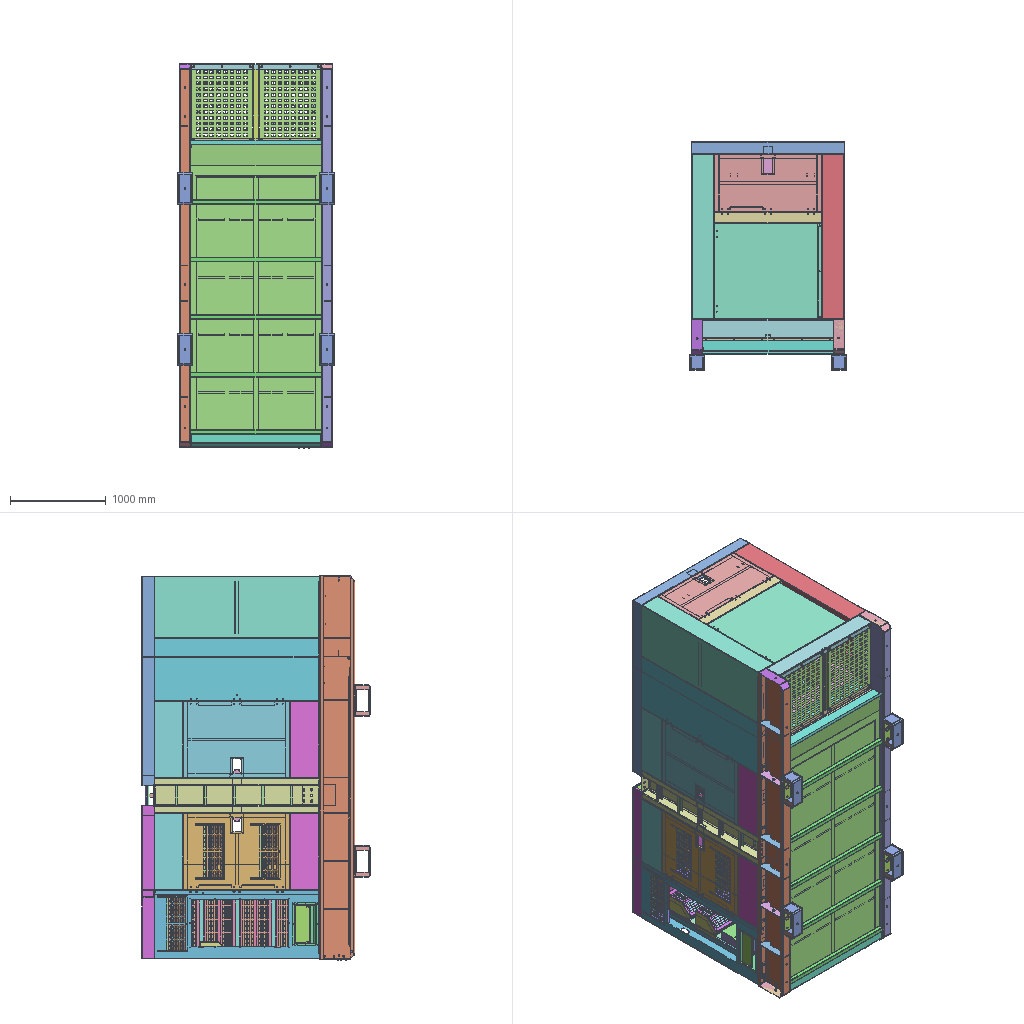Assembly | STEP file | 182 different items | 575 placed | box 1630 x 2379 x 4012 mm
Parts list (item | name | quantity | parent item | size | volume):
1 | 100 | x1 | in _X2_753574F68F8552A9652F67B6_X0_ASM | 200 x 40 x 280 mm | 410020 mm3
2 | 2290KW0001 | x1 | in VD-392-290KW00_ASM | 110 x 46 x 190 mm | 124105 mm3
3 | 290KW0001 | x1 | in VD-392-290KW00_ASM | 110 x 46 x 190 mm | 124105 mm3
4 | 3_1_00 | x1 | in 260_X2_975997F37535673A6A2A6881_ASM | - | -
5 | 3_2_00 | x1 | in 260_X2_975997F37535673A6A2A6881_ASM | 6 x 85 x 194 mm | 97590 mm3
6 | 400 | x1 | in 260_X2_975997F37535673A6A2A6881_ASM | 88 x 86 x 8 mm | 58744 mm3
7 | A_SYL0380DJ1008_1_4-1_CHACHE_AS | x4 | - | 330 x 152 x 150 mm | 725143 mm3
8 | A_SYL0380DJ1008_1_4-2_CHACHE_AS | x4 | - | 330 x 150 x 8 mm | 376221 mm3
9 | A_SYL0380DJ1008_1_4-3_CHACHE_AS | x8 | - | 313 x 143 x 8 mm | 135272 mm3
10 | B_SYL0380DJ1006_2_23-2_STEP | x1 | in MEN_ASM_STEP_ASM | 60 x 25 x 952 mm | 191493 mm3
11 | B_SYL0380DJ1008_2_9_1-1_STEP | x1 | in B_SYL0380DJ1008_2_9_1_ASM_STEP_ASM | 1114 x 994 x 52 mm | 2704262 mm3
12 | HEXAGON_NUTS_WITH_FLANGE_GB_GB_ | x2 | - | 34.5 x 34.5 x 16 mm | 6844 mm3
13 | M12_GB13681_2_VD-SYL0380DJ1006_ | x4 | in VD-SYL0380DJ1006_1_1_1_ASM_VD-S_ASM | 20.785 x 18 x 10.8 mm | 2100 mm3
14 | M12_GB13681_VD-SYL0380DJ1006_1_ | x4 | in VD-SYL0380DJ1006_1_1_1_ASM_VD-S_ASM | - | -
15 | M6X16_GB5787_VD-SYL0380DJ1006_1 | x5 | in VD-SYL0380DJ1006_1_0_ASM_VD-392_ASM | 13.413 x 13.413 x 22.7 mm | 929.946 mm3
16 | M6_GB13681_3_2_VD-SYL0380DJ1006 | x5 | in VD-SYL0380DJ1006_1_3_ASM_VD-SYL_ASM | - | -
17 | M6_GB13681_3_VD-SYL0380DJ1006_1 | x5 | in VD-SYL0380DJ1006_1_3_ASM_VD-SYL_ASM | 11.547 x 10 x 5.2 mm | 338.387 mm3
18 | PRT0001 | x1 | in VD-392-290KW00_ASM | 110 x 46 x 190 mm | 124105 mm3
19 | PRT0002 | x1 | in VD-392-290KW00_ASM | 110 x 46 x 190 mm | 124105 mm3
20 | SOCKET_BUTTON_HEAD_SCREW_ISO_IS | x4 | in VD-SYL0392DJ1006_1_2_ASM_VD-SYL_ASM | 14.75 x 9.5 x 9.5 mm | 358.994 mm3
21 | SYL0380DJ1008_2_7_2_1-1_STEP | x1 | in SYL0380DJ1008_2_7_2_1_ASM_STEP_ASM | 20 x 252 x 167 mm | 62697 mm3
22 | SYL0380DJ1008_2_7_2_1-2_STEP | x1 | in SYL0380DJ1008_2_7_2_1_ASM_STEP_ASM | 167 x 252 x 200 mm | 194104 mm3
23 | SYL0380DJ1008_2_7_2_1-3_STEP | x1 | in SYL0380DJ1008_2_7_2_1_ASM_STEP_ASM | 20 x 252 x 167 mm | 62974 mm3
24 | SYL0380DJ1008_2_7_2_2-1_STEP | x1 | in SYL0380DJ1008_2_7_2_2_ASM_STEP_ASM | 196 x 204 x 10 mm | 88727 mm3
25 | SYL_0392D6J1SYL0380DJ10-1018359 | x10 | in SYL_0392D6J1SYL0380DJ100-647163_ASM | 50 x 30 x 207 mm | 59466 mm3
26 | SYL_0392D6J1SYL0380DJ10-1066459 | x9 | in SYL_0392D6J1SYL0380DJ10-1760845_ASM | 38.5 x 325.355 x 203.95 mm | 94811 mm3
27 | SYL_0392D6J1SYL0380DJ10-1081048 | x2 | in SYL_0392D6J1SYL0380DJ10-1033257_ASM, SYL_0392D6J1SYL0380DJ100-434037_ASM | 1488 x 40 x 25 mm | 247870 mm3
28 | SYL_0392D6J1SYL0380DJ10-1098076 | x1 | in SYL_0392D6J1SYL0380DJ100-101261_ASM | 22 x 292 x 104 mm | 44923 mm3
29 | SYL_0392D6J1SYL0380DJ10-1103933 | x24 | in SYL_0392D6J1SYL0380DJ10-1255244_ASM, SYL_0392D6J1SYL0380DJ10-1517080_ASM, SYL_0392D6J1SYL0380DJ100-467540_ASM, SYL_0392D6J1SYL0380DJ100-774689_ASM, SYL_0392D6J1SYL0380DJ100-857854_ASM, SYL_0392D6J1SYL0380DJ100-948147_ASM | 1.5 x 45 x 300 mm | 17824 mm3
30 | SYL_0392D6J1SYL0380DJ10-1155504 | x1 | in SYL_0392D6J1SYL0380DJ100-948561_ASM | 794 x 1114 x 35 mm | 1839649 mm3
31 | SYL_0392D6J1SYL0380DJ10-1158695 | x1 | in SYL_0392D6J1SYL0380DJ100-994359_ASM | 1120 x 190 x 55 mm | 680109 mm3
32 | SYL_0392D6J1SYL0380DJ10-1205588 | x5 | in SYL_0392D6J1SYL0380DJ100-172504_ASM, SYL_0392D6J1SYL0380DJ100-972219_ASM | 38 x 20 x 458 mm | 46808 mm3
33 | SYL_0392D6J1SYL0380DJ10-1206392 | x1 | in SYL_0392D6J1SYL0380DJ100-591204_ASM | - | 2976644 mm3
34 | SYL_0392D6J1SYL0380DJ10-1266534 | x4 | in SYL_0392D6J1SYL0380DJ10-1033257_ASM, SYL_0392D6J1SYL0380DJ100-434037_ASM | 1586 x 125 x 30 mm | 300199 mm3
35 | SYL_0392D6J1SYL0380DJ10-1310194 | x2 | in SYL_0392D6J1SYL0380DJ10-1255244_ASM, SYL_0392D6J1SYL0380DJ100-774689_ASM | 50 x 35 x 1715 mm | 736400 mm3
36 | SYL_0392D6J1SYL0380DJ10-1332741 | x2 | in SYL_0392D6J1SYL0380DJ100-601081_ASM | 794 x 1114 x 35 mm | 2143366 mm3
37 | SYL_0392D6J1SYL0380DJ10-1341050 | x2 | in SYL_0392D6J1SYL0380DJ100-842586_ASM, SYL_0392D6J1SYL0380DJ100-948561_ASM | 30 x 25 x 525 mm | 76794 mm3
38 | SYL_0392D6J1SYL0380DJ10-1343368 | x5 | in SYL_0392D6J1SYL0380DJ100-172504_ASM, SYL_0392D6J1SYL0380DJ100-972219_ASM | 38 x 20 x 458 mm | 46807 mm3
39 | SYL_0392D6J1SYL0380DJ10-1361819 | x1 | in SYL_0392D6J1SYL0380DJ100-434037_ASM | 100 x 80 x 53 mm | 66751 mm3
40 | SYL_0392D6J1SYL0380DJ10-1368501 | x1 | in SYL_0392D6J1SYL0380DJ10-1695241_ASM | 370 x 160 x 2 mm | 38497 mm3
41 | SYL_0392D6J1SYL0380DJ10-1409429 | x2 | in SYL_0392D6J1SYL0380DJ100-857854_ASM, SYL_0392D6J1SYL0380DJ100-948147_ASM | 55 x 53 x 1714 mm | 657582 mm3
42 | SYL_0392D6J1SYL0380DJ10-1470572 | x3 | in SYL_0392D6J1SYL0380DJ100-357952_ASM, SYL_0392D6J1SYL0380DJ100-601081_ASM | 30 x 25 x 1018 mm | 149191 mm3
43 | SYL_0392D6J1SYL0380DJ10-1504831 | x4 | in SYL_0392D6J1SYL0380DJ1006_2-330_ASM | 144.153 x 95 x 24.659 mm | 58803 mm3
44 | SYL_0392D6J1SYL0380DJ10-1506056 | x1 | in SYL_0392D6J1SYL0380DJ100-413990_ASM | 40 x 53 x 10 mm | 21183 mm3
45 | SYL_0392D6J1SYL0380DJ10-1531669 | x1 | in SYL_0392D6J1SYL0380DJ10-1033257_ASM | 1585 x 77.2 x 123.6 mm | 1073180 mm3
46 | SYL_0392D6J1SYL0380DJ10-1554045 | x1 | in SYL_0392D6J1SYL0380DJ10-1695241_ASM | 370 x 160 x 3 mm | 158695 mm3
47 | SYL_0392D6J1SYL0380DJ10-1575320 | x1 | in SYL_0392D6J1SYL0380DJ10-1255244_ASM | 755 x 256 x 1738 mm | 2626332 mm3
48 | SYL_0392D6J1SYL0380DJ10-1577336 | x2 | in SYL_0392D6J1SYL0380DJ10-1566718_ASM | 125 x 964 x 292 mm | 507408 mm3
49 | SYL_0392D6J1SYL0380DJ10-1609202 | x2 | in SYL_0392D6J1SYL0380DJ100-357952_ASM | 80 x 33 x 30 mm | 15352 mm3
50 | SYL_0392D6J1SYL0380DJ10-1672638 | x2 | in SYL_0392D6J1SYL0380DJ10-1566718_ASM | 40.5 x 307.355 x 173.95 mm | 81571 mm3
51 | SYL_0392D6J1SYL0380DJ10-1680959 | x8 | in SYL_0392D6J1SYL0380DJ100-647163_ASM | 67.5 x 46.5 x 6 mm | 18616 mm3
52 | SYL_0392D6J1SYL0380DJ10-1703808 | x8 | in SYL_0392D6J1SYL0380DJ100-601081_ASM, SYL_0392D6J1SYL0380DJ100-842586_ASM, SYL_0392D6J1SYL0380DJ100-948561_ASM | 45 x 30 x 788 mm | 112936 mm3
53 | SYL_0392D6J1SYL0380DJ10-1713006 | x1 | - | 1478 x 1718 x 55 mm | 3668328 mm3
54 | SYL_0392D6J1SYL0380DJ10-1718718 | x2 | in SYL_0392D6J1SYL0380DJ10-1517080_ASM, SYL_0392D6J1SYL0380DJ100-467540_ASM | 40 x 27 x 550 mm | 95966 mm3
55 | SYL_0392D6J1SYL0380DJ10-1725835 | x2 | in SYL_0392D6J1SYL0380DJ100-357952_ASM | 44.9 x 29.9 x 588 mm | 79950 mm3
56 | SYL_0392D6J1SYL0380DJ100-138538 | x9 | in SYL_0392D6J1SYL0380DJ10-1760845_ASM | 38.5 x 325.355 x 203.95 mm | 94811 mm3
57 | SYL_0392D6J1SYL0380DJ100-148816 | x2 | in SYL_0392D6J1SYL0380DJ100-647163_ASM | 150 x 233 x 150 mm | 363200 mm3
58 | SYL_0392D6J1SYL0380DJ100-149154 | x9 | in SYL_0392D6J1SYL0380DJ100-520352_ASM | 550 x 152.382 x 325.821 mm | 213564 mm3
59 | SYL_0392D6J1SYL0380DJ100-161824 | x2 | in SYL_0392D6J1SYL0380DJ10-1566718_ASM | 40.5 x 307.355 x 173.95 mm | 81571 mm3
60 | SYL_0392D6J1SYL0380DJ100-163725 | x1 | in SYL_0392D6J1SYL0380DJ100-434037_ASM | - | 7732310 mm3
61 | SYL_0392D6J1SYL0380DJ100-170263 | x2 | in SYL_0392D6J1SYL0380DJ100-541371_ASM | 964 x 122.208 x 308.622 mm | 430080 mm3
62 | SYL_0392D6J1SYL0380DJ100-207422 | x3 | in SYL_0392D6J1SYL0380DJ10-1255244_ASM, SYL_0392D6J1SYL0380DJ100-774689_ASM | 1.5 x 45 x 100 mm | 5887 mm3
63 | SYL_0392D6J1SYL0380DJ100-232734 | x1 | in SYL_0392D6J1SYL0380DJ10-1033257_ASM | 1604 x 1592 x 165 mm | 6912474 mm3
64 | SYL_0392D6J1SYL0380DJ100-288319 | x5 | in SYL_0392D6J1SYL0380DJ100-357952_ASM, SYL_0392D6J1SYL0380DJ100-601081_ASM, SYL_0392D6J1SYL0380DJ100-842586_ASM, SYL_0392D6J1SYL0380DJ100-948561_ASM | 45 x 30 x 438 mm | 65045 mm3
65 | SYL_0392D6J1SYL0380DJ100-324063 | x9 | in SYL_0392D6J1SYL0380DJ10-1760845_ASM | 10 x 120 x 550 mm | 111077 mm3
66 | SYL_0392D6J1SYL0380DJ100-373455 | x4 | - | 804 x 343 x 55 mm | 764236 mm3
67 | SYL_0392D6J1SYL0380DJ100-382410 | x1 | in SYL_0392D6J1SYL0380DJ10-1517080_ASM | 650 x 1720 x 271 mm | 3661344 mm3
68 | SYL_0392D6J1SYL0380DJ100-399186 | x3 | in SYL_0392D6J1SYL0380DJ10-1179946_ASM, SYL_0392D6J1SYL0380DJ100-100350_ASM | 60 x 25 x 984 mm | 197947 mm3
69 | SYL_0392D6J1SYL0380DJ100-463198 | x8 | in SYL_0392D6J1SYL0380DJ100-972219_ASM | 38 x 20 x 740 mm | 74841 mm3
70 | SYL_0392D6J1SYL0380DJ100-474592 | x1 | in SYL_0392D6J1SYL0380DJ100-101261_ASM | 104 x 964 x 292 mm | 494830 mm3
71 | SYL_0392D6J1SYL0380DJ100-509338 | x2 | in SYL_0392D6J1SYL0380DJ100-647163_ASM | 360 x 1720 x 116 mm | 2326714 mm3
72 | SYL_0392D6J1SYL0380DJ100-519976 | x4 | in SYL_0392D6J1SYL0380DJ100-647163_ASM | 41 x 47 x 1707 mm | 289245 mm3
73 | SYL_0392D6J1SYL0380DJ100-542858 | x5 | in SYL_0392D6J1SYL0380DJ100-357952_ASM, SYL_0392D6J1SYL0380DJ100-601081_ASM, SYL_0392D6J1SYL0380DJ100-842586_ASM, SYL_0392D6J1SYL0380DJ100-948561_ASM | 45 x 30 x 438 mm | 65045 mm3
74 | SYL_0392D6J1SYL0380DJ100-543650 | x2 | in SYL_0392D6J1SYL0380DJ100-172504_ASM | 38 x 20 x 540 mm | 53472 mm3
75 | SYL_0392D6J1SYL0380DJ100-567986 | x1 | in SYL_0392D6J1SYL0380DJ100-774689_ASM | - | 3380150 mm3
76 | SYL_0392D6J1SYL0380DJ100-571255 | x1 | in SYL_0392D6J1SYL0380DJ10-1695241_ASM | 392 x 30.392 x 152.732 mm | 143186 mm3
77 | SYL_0392D6J1SYL0380DJ100-598208 | x1 | in SYL_0392D6J1SYL0380DJ100-948147_ASM | 1738 x 689 x 55 mm | 2865298 mm3
78 | SYL_0392D6J1SYL0380DJ100-608900 | x1 | in SYL_0392D6J1SYL0380DJ100-857854_ASM | 1738 x 689 x 55 mm | 2865327 mm3
79 | SYL_0392D6J1SYL0380DJ100-623151 | x1 | in SYL_0392D6J1SYL0380DJ100-357952_ASM | 594 x 1114 x 35 mm | 1655026 mm3
80 | SYL_0392D6J1SYL0380DJ100-648764 | x5 | in SYL_0392D6J1SYL0380DJ100-172504_ASM, SYL_0392D6J1SYL0380DJ100-972219_ASM | 38 x 20 x 1060 mm | 109009 mm3
81 | SYL_0392D6J1SYL0380DJ100-657039 | x2 | in SYL_0392D6J1SYL0380DJ10-1494631_ASM, SYL_0392D6J1SYL0380DJ10-1784118_ASM | 60 x 25 x 491 mm | 98000 mm3
82 | SYL_0392D6J1SYL0380DJ100-657963 | x1 | in SYL_0392D6J1SYL0380DJ100-101261_ASM | 22 x 292 x 104 mm | 44923 mm3
83 | SYL_0392D6J1SYL0380DJ100-674343 | x1 | in SYL_0392D6J1SYL0380DJ100-467540_ASM | 50 x 220 x 50 mm | 30996 mm3
84 | SYL_0392D6J1SYL0380DJ100-694871 | x1 | in SYL_0392D6J1SYL0380DJ100-413990_ASM | 40 x 250 x 40 mm | 314159 mm3
85 | SYL_0392D6J1SYL0380DJ100-698449 | x1 | in SYL_0392D6J1SYL0380DJ10-1069759_ASM | 446 x 269.609 x 269.8 mm | 707479 mm3
86 | SYL_0392D6J1SYL0380DJ100-774312 | x1 | in SYL_0392D6J1SYL0380DJ100-413990_ASM | 394.569 x 123 x 1592 mm | 1976035 mm3
87 | SYL_0392D6J1SYL0380DJ100-784216 | x5 | in SYL_0392D6J1SYL0380DJ10-1179946_ASM, SYL_0392D6J1SYL0380DJ10-1494631_ASM, SYL_0392D6J1SYL0380DJ10-1784118_ASM, SYL_0392D6J1SYL0380DJ100-100350_ASM | 49.95 x 167 x 223.5 mm | 65855 mm3
88 | SYL_0392D6J1SYL0380DJ100-786638 | x1 | in SYL_0392D6J1SYL0380DJ100-842586_ASM | 794 x 1114 x 35 mm | 1839812 mm3
89 | SYL_0392D6J1SYL0380DJ100-794406 | x1 | in SYL_0392D6J1SYL0380DJ100-434037_ASM | 1586 x 127 x 55 mm | 1040042 mm3
90 | SYL_0392D6J1SYL0380DJ100-808646 | x2 | in SYL_0392D6J1SYL0380DJ10-1179946_ASM | 30 x 50 x 80 mm | 20061 mm3
91 | SYL_0392D6J1SYL0380DJ100-884005 | x4 | in SYL0380DJ1008_2_7_2_1_ASM_STEP_ASM, SYL_0392D6J1SYL0380DJ10-1069759_ASM | 24 x 25 x 2 mm | 1062 mm3
92 | SYL_0392D6J1SYL0380DJ100-914702 | x1 | in SYL_0392D6J1SYL0380DJ100-973021_ASM | 1150 x 435 x 55 mm | 1345011 mm3
93 | SYL_0392D6J1SYL0380DJ100-939135 | x9 | in SYL_0392D6J1SYL0380DJ10-1760845_ASM | 155 x 550 x 310 mm | 314616 mm3
94 | SYL_0392D6J1SYL0380DJ100-987263 | x1 | in SYL_0392D6J1SYL0380DJ100-467540_ASM | 650 x 271 x 1720 mm | 3661245 mm3
95 | SYL_0392D6J1SYL0380DJ1006-79820 | x4 | in SYL_0392D6J1SYL0380DJ100-413990_ASM | 20 x 240 x 20 mm | 75398 mm3
96 | SYL_0392D6J1SYL0380DJ1006-90462 | x4 | in SYL_0392D6J1SYL0380DJ100-647163_ASM | 100 x 65 x 49 mm | 49825 mm3
97 | SYL_0392D6J1SYL0380DJ1006-92088 | x7 | in SYL_0392D6J1SYL0380DJ100-357952_ASM, SYL_0392D6J1SYL0380DJ100-601081_ASM, SYL_0392D6J1SYL0380DJ100-948561_ASM | 45 x 30 x 345 mm | 53987 mm3
98 | SYL_0392D6J1SYL0380DJ1006_2_1-1 | x1 | in SYL_0392D6J1SYL0380DJ1006_2_1_A_ASM | 224 x 212 x 52 mm | 119868 mm3
99 | SYL_0392D6J1SYL0380DJ1006_2_1-2 | x2 | in SYL_0392D6J1SYL0380DJ1006_2_1_A_ASM, SYL_0392D6J1SYL0380DJ1006_2_2_A_ASM | 84 x 25 x 550 mm | 136985 mm3
100 | SYL_0392D6J1SYL0380DJ1006_2_11- | x3 | - | 800 x 335 x 53 mm | 743196 mm3
101 | SYL_0392D6J1SYL0380DJ1006_2_11X | x1 | in SYL_0392D6J1MK1_STEP_ASM | 800 x 335 x 53 mm | 648025 mm3
102 | SYL_0392D6J1SYL0380DJ1006_2_5-1 | x2 | in SYL_0392D6J1SYL0380DJ1006_2_5_A_ASM, SYL_0392D6J1SYL0380DJ1006_2_6_A_ASM | 84 x 25 x 1478 mm | 368355 mm3
103 | SYL_0392D6J1SYL0380DJ1006_2_5-2 | x3 | in SYL_0392D6J1SYL0380DJ1006_2_5_A_ASM | 44 x 4.447 x 500 mm | 32801 mm3
104 | SYL_0392D6J1SYL0380DJ1006_2_6-1 | x4 | in SYL_0392D6J1SYL0380DJ1006_2_6_A_ASM | 44 x 4.447 x 200 mm | 12970 mm3
105 | SYL_0392D6J1SYL0380DJ1006_2_6-5 | x1 | in SYL_0392D6J1SYL0380DJ1006_2_6_A_ASM | 30 x 90 x 80 mm | 26496 mm3
106 | - | x5 | in SYL_0392D6J1SYL0380DJ100-434037_ASM | 40 x 120 x 8 mm | 37600 mm3
107 | VD-120102160011A_1_STEP | x8 | in VD-SYL0380DJ1006_1_2_1_ASM_STEP_ASM | 16.166 x 14 x 6.5 mm | 760.223 mm3
108 | VD-120102160011A_1_VD-SY-325206 | x21 | in VD-SYL0380DJ1006_1_1_ASM_VD-SYL_ASM | 16.166 x 14 x 6.5 mm | 760.223 mm3
109 | VD-120102160011A_1_VD-SY-452498 | x6 | in VD-SYL0380DJ1006_1_3_ASM_VD-SYL_ASM | 16.166 x 14 x 6.5 mm | 760.223 mm3
110 | VD-120102160011A_1_VD-SY-509251 | x2 | in VD-SYL0380DJ1006_1_1_4_ASM_VD-S_ASM | 16.166 x 14 x 6.5 mm | 760.223 mm3
111 | VD-120102160011A_1_VD-SYL-80020 | x10 | in VD-SYL0380DJ1006_1_1_2_ASM_VD-S_ASM | 16.166 x 14 x 6.5 mm | 760.223 mm3
112 | VD-120102160011A_1_VD-SYL0-5601 | x8 | in VD-SYL0380DJ1006_1_1_1_ASM_VD-S_ASM | 16.166 x 14 x 6.5 mm | 760.223 mm3
113 | VD-151208000366A_DN15_X2_76F490 | x2 | - | 26 x 26 x 26 mm | 9182 mm3
114 | VD-60063402_1_2_VD-SYL03-211777 | x36 | in VD-SYL0380DJ1006_1_0_ASM_VD-392_ASM | - | -
115 | VD-60063402_1_VD-SYL0380-322120 | x38 | in VD-SYL0380DJ1006_1_0_ASM_VD-392_ASM | 19.856 x 33.5 x 19.856 mm | 2596 mm3
116 | VD-J260_10_1_1A_1-20_2_VD-SYL03 | x1 | in VD-SYL0380DJ1006_1_1_ASM_VD-SYL_ASM | - | -
117 | VD-J260_10_1_1A_1-20_VD-SYL0380 | x1 | in VD-SYL0380DJ1006_1_1_ASM_VD-SYL_ASM | 25 x 20 x 25 mm | 8673 mm3
118 | VD-SYL0380DJ1006_1-1_VD-SYL0380 | x1 | in VD-SYL0380DJ1006_1_0_ASM_VD-392_ASM | 70 x 350 x 160 mm | 388659 mm3
119 | VD-SYL0380DJ1006_1-2_VD-SYL0380 | x1 | in VD-SYL0380DJ1006_1_0_ASM_VD-392_ASM | 60 x 40 x 1470 mm | 567408 mm3
120 | VD-SYL0380DJ1006_1-3_VD-SYL0380 | x1 | in VD-SYL0380DJ1006_1_0_ASM_VD-392_ASM | 130 x 122.663 x 5 mm | 63619 mm3
121 | VD-SYL0380DJ1006_1-4_VD-SYL0380 | x4 | in VD-SYL0380DJ1006_1_0_ASM_VD-392_ASM | 108 x 41 x 35 mm | 12075 mm3
122 | VD-SYL0380DJ1006_1-5_VD-SYL0380 | x2 | in VD-SYL0380DJ1006_1_0_ASM_VD-392_ASM | 630 x 805 x 2 mm | 782388 mm3
123 | VD-SYL0380DJ1006_1-6_VD-SYL0380 | x1 | in VD-SYL0380DJ1006_1_0_ASM_VD-392_ASM | - | -
124 | VD-SYL0380DJ1006_1-7_VD-SYL0380 | x1 | in VD-SYL0380DJ1006_1_0_ASM_VD-392_ASM | - | -
125 | VD-SYL0380DJ1006_1-8_VD-SYL0380 | x1 | in VD-SYL0380DJ1006_1_0_ASM_VD-392_ASM | 185 x 140 x 50 mm | 149401 mm3
126 | VD-SYL0380DJ1006_1-9_VD-SYL0380 | x1 | in VD-SYL0380DJ1006_1_0_ASM_VD-392_ASM | 100 x 30 x 80 mm | 27724 mm3
127 | VD-SYL0380DJ1006_1_1-10_VD-SYL0 | x1 | in VD-SYL0380DJ1006_1_1_ASM_VD-SYL_ASM | 1360 x 25 x 60 mm | 325121 mm3
128 | VD-SYL0380DJ1006_1_1-11_VD-SYL0 | x2 | in VD-SYL0380DJ1006_1_1_ASM_VD-SYL_ASM | 220 x 350 x 16 mm | 1185235 mm3
129 | VD-SYL0380DJ1006_1_1-12_VD-SYL0 | x2 | in VD-SYL0380DJ1006_1_1_ASM_VD-SYL_ASM | 300 x 60 x 80 mm | 184401 mm3
130 | VD-SYL0380DJ1006_1_1-13_VD-SYL0 | x1 | in VD-SYL0380DJ1006_1_1_ASM_VD-SYL_ASM | 60 x 30 x 830 mm | 274242 mm3
131 | VD-SYL0380DJ1006_1_1-14_VD-SYL0 | x4 | in VD-SYL0380DJ1006_1_1_ASM_VD-SYL_ASM | 106 x 356 x 10 mm | 301941 mm3
132 | VD-SYL0380DJ1006_1_1-15_2_VD-SY | x3 | in VD-SYL0380DJ1006_1_1_ASM_VD-SYL_ASM | 28 x 28 x 50 mm | 17920 mm3
133 | VD-SYL0380DJ1006_1_1-15_VD-SYL0 | x3 | in VD-SYL0380DJ1006_1_1_ASM_VD-SYL_ASM | - | -
134 | VD-SYL0380DJ1006_1_1-3_VD-SYL03 | x1 | in VD-SYL0380DJ1006_1_1_ASM_VD-SYL_ASM | 50 x 1360 x 365 mm | 1816160 mm3
135 | VD-SYL0380DJ1006_1_1-4_VD-SYL03 | x1 | in VD-SYL0380DJ1006_1_1_ASM_VD-SYL_ASM | 200 x 1360 x 55 mm | 1991838 mm3
136 | VD-SYL0380DJ1006_1_1-5_VD-SYL03 | x5 | in VD-SYL0380DJ1006_1_1_ASM_VD-SYL_ASM | 1360 x 50 x 50 mm | 735519 mm3
137 | VD-SYL0380DJ1006_1_1-6_VD-SYL03 | x1 | in VD-SYL0380DJ1006_1_1_ASM_VD-SYL_ASM | 2999 x 1359 x 24.985 mm | 8157094 mm3
138 | VD-SYL0380DJ1006_1_1-7_VD-392-_ | x2 | - | - | -
139 | VD-SYL0380DJ1006_1_1-7_VD-SYL03 | x2 | in VD-SYL0380DJ1006_1_1_ASM_VD-SYL_ASM | 114 x 363.205 x 53.74 mm | 215041 mm3
140 | VD-SYL0380DJ1006_1_1-8_VD-SYL03 | x2 | in VD-SYL0380DJ1006_1_1_ASM_VD-SYL_ASM | - | -
141 | VD-SYL0380DJ1006_1_1-9_VD-SYL03 | x8 | in VD-SYL0380DJ1006_1_1_ASM_VD-SYL_ASM | 106 x 356 x 10 mm | 309009 mm3
142 | VD-SYL0380DJ1006_1_1_1-1_VD-SYL | x1 | in VD-SYL0380DJ1006_1_1_1_ASM_VD-S_ASM | 180 x 70 x 1450 mm | 2600657 mm3
143 | VD-SYL0380DJ1006_1_1_1-2-294573 | x1 | in VD-SYL0380DJ1006_1_1_1_ASM_VD-S_ASM | 1450 x 100 x 54 mm | 1690826 mm3
144 | VD-SYL0380DJ1006_1_1_1-2-492428 | x1 | in VD-SYL0380DJ1006_1_1_2_ASM_VD-S_ASM | 1450 x 100 x 54 mm | 1690826 mm3
145 | VD-SYL0380DJ1006_1_1_2-1_VD-SYL | x1 | in VD-SYL0380DJ1006_1_1_2_ASM_VD-S_ASM | 180 x 70 x 1450 mm | 2609055 mm3
146 | VD-SYL0380DJ1006_1_1_2-2_VD-SYL | x4 | in VD-SYL0380DJ1006_1_1_2_ASM_VD-S_ASM | 120 x 45 x 164 mm | 186599 mm3
147 | VD-SYL0380DJ1006_1_1_2-3_VD-SYL | x2 | in VD-SYL0380DJ1006_1_1_2_ASM_VD-S_ASM | 210 x 140 x 10 mm | 239785 mm3
148 | VD-SYL0380DJ1006_1_1_4-1_VD-SYL | x1 | in VD-SYL0380DJ1006_1_1_4_ASM_VD-S_ASM | 180 x 50 x 1360 mm | 2129804 mm3
149 | VD-SYL0380DJ1006_1_1_4-2_VD-SYL | x2 | in VD-SYL0380DJ1006_1_1_4_ASM_VD-S_ASM | 120 x 103 x 290 mm | 366206 mm3
150 | VD-SYL0380DJ1006_1_1_4-3_VD-SYL | x4 | in VD-SYL0380DJ1006_1_1_4_ASM_VD-S_ASM | 114 x 97 x 6 mm | 66240 mm3
151 | VD-SYL0380DJ1006_1_2_1-1_STEP | x1 | in VD-SYL0380DJ1006_1_2_1_ASM_STEP_ASM | 1300 x 267 x 2700 mm | 14741994 mm3
152 | VD-SYL0380DJ1006_1_2_1-2_STEP | x1 | in VD-SYL0380DJ1006_1_2_1_ASM_STEP_ASM | 1250 x 254 x 2680 mm | 11864231 mm3
153 | VD-SYL0380DJ1006_1_2_1-3_STEP | x4 | in VD-SYL0380DJ1006_1_2_1_ASM_STEP_ASM | 25 x 251 x 1248 mm | 994019 mm3
154 | VD-SYL0380DJ1006_1_2_1-4_STEP | x4 | in VD-SYL0380DJ1006_1_2_1_ASM_STEP_ASM | 10 x 50 x 100 mm | 28966 mm3
155 | VD-SYL0380DJ1006_1_2_1-5_STEP | x1 | in VD-SYL0380DJ1006_1_2_1_ASM_STEP_ASM | 2672 x 40 x 40 mm | 1124439 mm3
156 | VD-SYL0380DJ1006_1_2_1-6_STEP | x1 | in VD-SYL0380DJ1006_1_2_1_ASM_STEP_ASM | 50 x 25 x 2672 mm | 722540 mm3
157 | VD-SYL0380DJ1006_1_2_1-9_2_DN15 | x2 | - | 28 x 28 x 25 mm | 8888 mm3
158 | VD-SYL0380DJ1006_1_2_1-9_2_STEP | x1 | in VD-SYL0380DJ1006_1_2_1_ASM_STEP_ASM | 28 x 28 x 25 mm | 8888 mm3
159 | VD-SYL0380DJ1006_1_2_1-9_STEP | x1 | in VD-SYL0380DJ1006_1_2_1_ASM_STEP_ASM | - | -
160 | VD-SYL0380DJ1006_1_3-1_VD-SYL03 | x1 | in VD-SYL0380DJ1006_1_3_ASM_VD-SYL_ASM | 1354 x 132 x 353 mm | 2119091 mm3
161 | VD-SYL0380DJ1006_1_4-1_VD-SYL03 | x2 | in VD-SYL0380DJ1006_1_4_ASM_VD-SYL_ASM | 92.5 x 167 x 140 mm | 350886 mm3
162 | VD-SYL0380DJ1006_1_4-2_VD-SYL03 | x2 | in VD-SYL0380DJ1006_1_4_ASM_VD-SYL_ASM | 10 x 70 x 120 mm | 57804 mm3
163 | VD-SYL0380DJ1006_1_4-3_VD-SYL03 | x4 | in VD-SYL0380DJ1006_1_4_ASM_VD-SYL_ASM | 10 x 80 x 249 mm | 187272 mm3
164 | VD-SYL0380DJ1006_1_4-4_VD-SYL03 | x2 | in VD-SYL0380DJ1006_1_4_ASM_VD-SYL_ASM | 10 x 130 x 80 mm | 99265 mm3
165 | VD-SYL0380DJ1006_1_4-5_VD-SYL03 | x2 | in VD-SYL0380DJ1006_1_4_ASM_VD-SYL_ASM | 94 x 65.818 x 249 mm | 245764 mm3
166 | VD-SYL0380DJ1006_1_5-1_VD-SYL03 | x2 | in VD-SYL0380DJ1006_1_5_ASM_VD-SYL_ASM | 110 x 93 x 230 mm | 284786 mm3
167 | VD-SYL0380DJ1006_1_5-2_VD-SYL03 | x2 | in VD-SYL0380DJ1006_1_5_ASM_VD-SYL_ASM | 10 x 70 x 95 mm | 46554 mm3
168 | VD-SYL0380DJ1006_1_5-3_VD-SYL03 | x4 | in VD-SYL0380DJ1006_1_5_ASM_VD-SYL_ASM | 10 x 80 x 190 mm | 124687 mm3
169 | VD-SYL0380DJ1006_1_5-4_VD-SYL03 | x2 | in VD-SYL0380DJ1006_1_5_ASM_VD-SYL_ASM | 10 x 103 x 80 mm | 77665 mm3
170 | VD-SYL0380DJ1006_1_5-5_VD-SYL03 | x2 | in VD-SYL0380DJ1006_1_5_ASM_VD-SYL_ASM | 73 x 83.716 x 190 mm | 151290 mm3
171 | VD-SYL0392DJ1006_1_1-1_VD-SYL03 | x1 | in VD-SYL0380DJ1006_1_1_ASM_VD-SYL_ASM | 120 x 370 x 4000 mm | 15499432 mm3
172 | VD-SYL0392DJ1006_1_1-2_VD-SYL03 | x1 | in VD-SYL0380DJ1006_1_1_ASM_VD-SYL_ASM | 120 x 370 x 4000 mm | 15496824 mm3
173 | _10001 | x1 | in 260_X2_975997F37535673A6A2A6881_ASM | 240 x 93 x 210 mm | 700527 mm3
174 | _10002 | x1 | in 260_X2_975997F37535673A6A2A6881_ASM | 6 x 85 x 194 mm | 97590 mm3
175 | _20001 | x1 | in 260_X2_975997F37535673A6A2A6881_ASM | 210 x 100 x 1450 mm | 3332053 mm3
176 | _20002 | x1 | in 260_X2_975997F37535673A6A2A6881_ASM | 100 x 94 x 1450 mm | 1590791 mm3
177 | _30001 | x1 | in 260_X2_975997F37535673A6A2A6881_ASM | 6 x 88 x 1450 mm | 765600 mm3
178 | _50001 | x1 | in 260_X2_975997F37535673A6A2A6881_ASM | 88 x 88 x 8 mm | 60152 mm3
179 | _HEXAGON_WELD_NUTS_GB_-_-257103 | x1 | in _X2_753574F68F8552A9652F67B6_X0_ASM | 21.939 x 10 x 19 mm | 1991 mm3
180 | _HEXAGON_WELD_NUTS_GB_-_-378705 | x1 | in 260_X2_975997F37535673A6A2A6881_ASM | 16.166 x 6.5 x 14 mm | 760.254 mm3
181 | _HEXAGON_WELD_NUTS_GB_-_-508666 | x1 | in _X2_753574F68F8552A9652F67B6_X0_ASM | 21.939 x 10 x 19 mm | 1991 mm3
182 | _HEXAGON_WELD_NUTS_GB_-_E-25802 | x1 | in 260_X2_975997F37535673A6A2A6881_ASM | 16.166 x 6.5 x 14 mm | 760.254 mm3